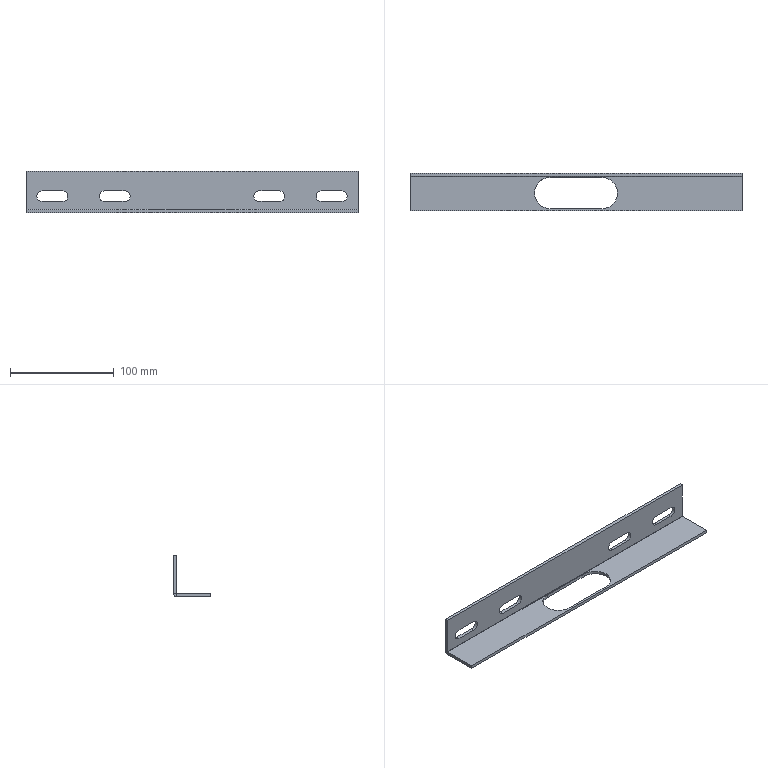Part | SolidWorks | features Cut 2, EdgeFlange 1, FlatPattern 1, SMBaseFlange 1, SheetMetal 1 | 1 solid | 35 faces | box 320 x 36 x 40 mm | volume 59416 mm3 | plane 22 | cylinder 13 | commonest cylinder face diameters 10 x8 30 x3 0.4 x1 6.4 x1
STEP:
#1=CARTESIAN_POINT('',(40.,-1.,-3.));
#2=VERTEX_POINT('',#1);
#3=CARTESIAN_POINT('',(25.,14.,-3.));
#4=VERTEX_POINT('',#3);
#5=CARTESIAN_POINT('',(25.,-1.,-3.));
#6=DIRECTION('',(0.,0.,1.));
#7=DIRECTION('',(1.,0.,0.));
#8=AXIS2_PLACEMENT_3D('',#5,#6,#7);
#9=CIRCLE('',#8,15.);
#10=EDGE_CURVE('',#2,#4,#9,.T.);
#11=ORIENTED_EDGE('',*,*,#10,.F.);
#12=CARTESIAN_POINT('',(40.,-1.,0.));
#13=VERTEX_POINT('',#12);
#14=CARTESIAN_POINT('',(40.,-1.,-10.));
#15=DIRECTION('',(0.,0.,1.));
#16=VECTOR('',#15,1000.);
#17=LINE('',#14,#16);
#18=EDGE_CURVE('',#2,#13,#17,.T.);
#19=ORIENTED_EDGE('',*,*,#18,.T.);
#20=CARTESIAN_POINT('',(25.,14.,0.));
#21=VERTEX_POINT('',#20);
#22=CARTESIAN_POINT('',(25.,-1.,0.));
#23=DIRECTION('',(0.,0.,1.));
#24=DIRECTION('',(1.,0.,0.));
#25=AXIS2_PLACEMENT_3D('',#22,#23,#24);
#26=CIRCLE('',#25,15.);
#27=EDGE_CURVE('',#13,#21,#26,.T.);
#28=ORIENTED_EDGE('',*,*,#27,.T.);
#29=CARTESIAN_POINT('',(25.,14.,-10.));
#30=DIRECTION('',(0.,0.,1.));
#31=VECTOR('',#30,1000.);
#32=LINE('',#29,#31);
#33=EDGE_CURVE('',#4,#21,#32,.T.);
#34=ORIENTED_EDGE('',*,*,#33,.F.);
#35=EDGE_LOOP('',(#11,#19,#28,#34));
#36=FACE_OUTER_BOUND('',#35,.T.);
#37=CARTESIAN_POINT('',(25.,-1.,-10.));
#38=DIRECTION('',(0.,0.,1.));
#39=DIRECTION('',(1.,0.,0.));
#40=AXIS2_PLACEMENT_3D('',#37,#38,#39);
#41=CYLINDRICAL_SURFACE('',#40,15.);
#42=ADVANCED_FACE('',(#36),#41,.F.);
#43=CARTESIAN_POINT('',(-160.,14.8,0.));
#44=VERTEX_POINT('',#43);
#45=CARTESIAN_POINT('',(-160.,-18.,0.));
#46=VERTEX_POINT('',#45);
#47=CARTESIAN_POINT('',(-160.,18.,0.));
#48=DIRECTION('',(0.,-1.,0.));
#49=VECTOR('',#48,1000.);
#50=LINE('',#47,#49);
#51=EDGE_CURVE('',#44,#46,#50,.T.);
#52=ORIENTED_EDGE('',*,*,#51,.F.);
#53=CARTESIAN_POINT('',(-160.,14.8,-3.));
#54=VERTEX_POINT('',#53);
#55=CARTESIAN_POINT('',(-160.,14.8,0.));
#56=DIRECTION('',(0.,0.,-1.));
#57=VECTOR('',#56,1000.);
#58=LINE('',#55,#57);
#59=EDGE_CURVE('',#44,#54,#58,.T.);
#60=ORIENTED_EDGE('',*,*,#59,.T.);
#61=CARTESIAN_POINT('',(-160.,-18.,-3.));
#62=VERTEX_POINT('',#61);
#63=CARTESIAN_POINT('',(-160.,18.,-3.));
#64=DIRECTION('',(0.,-1.,0.));
#65=VECTOR('',#64,1000.);
#66=LINE('',#63,#65);
#67=EDGE_CURVE('',#54,#62,#66,.T.);
#68=ORIENTED_EDGE('',*,*,#67,.T.);
#69=CARTESIAN_POINT('',(-160.,-18.,-3.));
#70=DIRECTION('',(0.,0.,1.));
#71=VECTOR('',#70,1000.);
#72=LINE('',#69,#71);
#73=EDGE_CURVE('',#62,#46,#72,.T.);
#74=ORIENTED_EDGE('',*,*,#73,.T.);
#75=EDGE_LOOP('',(#52,#60,#68,#74));
#76=FACE_OUTER_BOUND('',#75,.T.);
#77=CARTESIAN_POINT('',(-160.,18.,-3.));
#78=DIRECTION('',(-1.,0.,0.));
#79=DIRECTION('',(0.,0.,1.));
#80=AXIS2_PLACEMENT_3D('',#77,#78,#79);
#81=PLANE('',#80);
#82=ADVANCED_FACE('',(#76),#81,.T.);
#83=CARTESIAN_POINT('',(-25.,14.,-3.));
#84=VERTEX_POINT('',#83);
#85=CARTESIAN_POINT('',(0.,14.,-3.));
#86=DIRECTION('',(-1.,0.,0.));
#87=VECTOR('',#86,1000.);
#88=LINE('',#85,#87);
#89=EDGE_CURVE('',#4,#84,#88,.T.);
#90=ORIENTED_EDGE('',*,*,#89,.T.);
#91=CARTESIAN_POINT('',(-25.,-16.,-3.));
#92=VERTEX_POINT('',#91);
#93=CARTESIAN_POINT('',(-25.,-1.,-3.));
#94=DIRECTION('',(0.,0.,1.));
#95=DIRECTION('',(1.,0.,0.));
#96=AXIS2_PLACEMENT_3D('',#93,#94,#95);
#97=CIRCLE('',#96,15.);
#98=EDGE_CURVE('',#84,#92,#97,.T.);
#99=ORIENTED_EDGE('',*,*,#98,.T.);
#100=CARTESIAN_POINT('',(25.,-16.,-3.));
#101=VERTEX_POINT('',#100);
#102=CARTESIAN_POINT('',(0.,-16.,-3.));
#103=DIRECTION('',(1.,0.,0.));
#104=VECTOR('',#103,1000.);
#105=LINE('',#102,#104);
#106=EDGE_CURVE('',#92,#101,#105,.T.);
#107=ORIENTED_EDGE('',*,*,#106,.T.);
#108=CARTESIAN_POINT('',(25.,-1.,-3.));
#109=DIRECTION('',(0.,0.,1.));
#110=DIRECTION('',(1.,0.,0.));
#111=AXIS2_PLACEMENT_3D('',#108,#109,#110);
#112=CIRCLE('',#111,15.);
#113=EDGE_CURVE('',#101,#2,#112,.T.);
#114=ORIENTED_EDGE('',*,*,#113,.T.);
#115=ORIENTED_EDGE('',*,*,#10,.T.);
#116=EDGE_LOOP('',(#90,#99,#107,#114,#115));
#117=FACE_BOUND('',#116,.T.);
#118=CARTESIAN_POINT('',(160.,14.8,-3.));
#119=VERTEX_POINT('',#118);
#120=CARTESIAN_POINT('',(-160.,14.8,-3.));
#121=DIRECTION('',(1.,0.,0.));
#122=VECTOR('',#121,1000.);
#123=LINE('',#120,#122);
#124=EDGE_CURVE('',#54,#119,#123,.T.);
#125=ORIENTED_EDGE('',*,*,#124,.T.);
#126=CARTESIAN_POINT('',(160.,-18.,-3.));
#127=VERTEX_POINT('',#126);
#128=CARTESIAN_POINT('',(160.,18.,-3.));
#129=DIRECTION('',(0.,1.,0.));
#130=VECTOR('',#129,1000.);
#131=LINE('',#128,#130);
#132=EDGE_CURVE('',#127,#119,#131,.T.);
#133=ORIENTED_EDGE('',*,*,#132,.F.);
#134=CARTESIAN_POINT('',(-160.,-18.,-3.));
#135=DIRECTION('',(1.,0.,0.));
#136=VECTOR('',#135,1000.);
#137=LINE('',#134,#136);
#138=EDGE_CURVE('',#62,#127,#137,.T.);
#139=ORIENTED_EDGE('',*,*,#138,.F.);
#140=ORIENTED_EDGE('',*,*,#67,.F.);
#141=EDGE_LOOP('',(#125,#133,#139,#140));
#142=FACE_OUTER_BOUND('',#141,.T.);
#143=CARTESIAN_POINT('',(0.,0.,-3.));
#144=DIRECTION('',(0.,0.,1.));
#145=DIRECTION('',(1.,0.,0.));
#146=AXIS2_PLACEMENT_3D('',#143,#144,#145);
#147=PLANE('',#146);
#148=ADVANCED_FACE('',(#117,#142),#147,.F.);
#149=CARTESIAN_POINT('',(-25.,14.,0.));
#150=VERTEX_POINT('',#149);
#151=CARTESIAN_POINT('',(-25.,-16.,0.));
#152=VERTEX_POINT('',#151);
#153=CARTESIAN_POINT('',(-25.,-1.,0.));
#154=DIRECTION('',(0.,0.,1.));
#155=DIRECTION('',(1.,0.,0.));
#156=AXIS2_PLACEMENT_3D('',#153,#154,#155);
#157=CIRCLE('',#156,15.);
#158=EDGE_CURVE('',#150,#152,#157,.T.);
#159=ORIENTED_EDGE('',*,*,#158,.F.);
#160=CARTESIAN_POINT('',(-25.,14.,0.));
#161=DIRECTION('',(-1.,0.,0.));
#162=VECTOR('',#161,1000.);
#163=LINE('',#160,#162);
#164=EDGE_CURVE('',#21,#150,#163,.T.);
#165=ORIENTED_EDGE('',*,*,#164,.F.);
#166=ORIENTED_EDGE('',*,*,#27,.F.);
#167=CARTESIAN_POINT('',(25.,-16.,0.));
#168=VERTEX_POINT('',#167);
#169=CARTESIAN_POINT('',(25.,-1.,0.));
#170=DIRECTION('',(0.,0.,1.));
#171=DIRECTION('',(1.,0.,0.));
#172=AXIS2_PLACEMENT_3D('',#169,#170,#171);
#173=CIRCLE('',#172,15.);
#174=EDGE_CURVE('',#168,#13,#173,.T.);
#175=ORIENTED_EDGE('',*,*,#174,.F.);
#176=CARTESIAN_POINT('',(-25.,-16.,0.));
#177=DIRECTION('',(1.,0.,0.));
#178=VECTOR('',#177,1000.);
#179=LINE('',#176,#178);
#180=EDGE_CURVE('',#152,#168,#179,.T.);
#181=ORIENTED_EDGE('',*,*,#180,.F.);
#182=EDGE_LOOP('',(#159,#165,#166,#175,#181));
#183=FACE_BOUND('',#182,.T.);
#184=CARTESIAN_POINT('',(160.,-18.,0.));
#185=VERTEX_POINT('',#184);
#186=CARTESIAN_POINT('',(160.,14.8,0.));
#187=VERTEX_POINT('',#186);
#188=CARTESIAN_POINT('',(160.,18.,0.));
#189=DIRECTION('',(0.,1.,0.));
#190=VECTOR('',#189,1000.);
#191=LINE('',#188,#190);
#192=EDGE_CURVE('',#185,#187,#191,.T.);
#193=ORIENTED_EDGE('',*,*,#192,.T.);
#194=CARTESIAN_POINT('',(-160.,14.8,0.));
#195=DIRECTION('',(1.,0.,0.));
#196=VECTOR('',#195,1000.);
#197=LINE('',#194,#196);
#198=EDGE_CURVE('',#44,#187,#197,.T.);
#199=ORIENTED_EDGE('',*,*,#198,.F.);
#200=ORIENTED_EDGE('',*,*,#51,.T.);
#201=CARTESIAN_POINT('',(-160.,-18.,0.));
#202=DIRECTION('',(1.,0.,0.));
#203=VECTOR('',#202,1000.);
#204=LINE('',#201,#203);
#205=EDGE_CURVE('',#46,#185,#204,.T.);
#206=ORIENTED_EDGE('',*,*,#205,.T.);
#207=EDGE_LOOP('',(#193,#199,#200,#206));
#208=FACE_OUTER_BOUND('',#207,.T.);
#209=CARTESIAN_POINT('',(0.,0.,0.));
#210=DIRECTION('',(0.,0.,1.));
#211=DIRECTION('',(1.,0.,0.));
#212=AXIS2_PLACEMENT_3D('',#209,#210,#211);
#213=PLANE('',#212);
#214=ADVANCED_FACE('',(#183,#208),#213,.T.);
#215=CARTESIAN_POINT('',(160.,14.8,0.));
#216=DIRECTION('',(0.,0.,-1.));
#217=VECTOR('',#216,1000.);
#218=LINE('',#215,#217);
#219=EDGE_CURVE('',#187,#119,#218,.T.);
#220=ORIENTED_EDGE('',*,*,#219,.F.);
#221=ORIENTED_EDGE('',*,*,#192,.F.);
#222=CARTESIAN_POINT('',(160.,-18.,-3.));
#223=DIRECTION('',(0.,0.,1.));
#224=VECTOR('',#223,1000.);
#225=LINE('',#222,#224);
#226=EDGE_CURVE('',#127,#185,#225,.T.);
#227=ORIENTED_EDGE('',*,*,#226,.F.);
#228=ORIENTED_EDGE('',*,*,#132,.T.);
#229=EDGE_LOOP('',(#220,#221,#227,#228));
#230=FACE_OUTER_BOUND('',#229,.T.);
#231=CARTESIAN_POINT('',(160.,18.,-3.));
#232=DIRECTION('',(1.,0.,0.));
#233=DIRECTION('',(0.,0.,-1.));
#234=AXIS2_PLACEMENT_3D('',#231,#232,#233);
#235=PLANE('',#234);
#236=ADVANCED_FACE('',(#230),#235,.T.);
#237=ORIENTED_EDGE('',*,*,#205,.F.);
#238=ORIENTED_EDGE('',*,*,#73,.F.);
#239=ORIENTED_EDGE('',*,*,#138,.T.);
#240=ORIENTED_EDGE('',*,*,#226,.T.);
#241=EDGE_LOOP('',(#237,#238,#239,#240));
#242=FACE_OUTER_BOUND('',#241,.T.);
#243=CARTESIAN_POINT('',(-160.,-18.,-3.));
#244=DIRECTION('',(0.,-1.,0.));
#245=DIRECTION('',(0.,0.,-1.));
#246=AXIS2_PLACEMENT_3D('',#243,#244,#245);
#247=PLANE('',#246);
#248=ADVANCED_FACE('',(#242),#247,.T.);
#249=CARTESIAN_POINT('',(160.,15.,0.2));
#250=VERTEX_POINT('',#249);
#251=CARTESIAN_POINT('',(160.,18.,0.2));
#252=VERTEX_POINT('',#251);
#253=CARTESIAN_POINT('',(160.,18.,0.2));
#254=DIRECTION('',(0.,1.,0.));
#255=VECTOR('',#254,1000.);
#256=LINE('',#253,#255);
#257=EDGE_CURVE('',#250,#252,#256,.T.);
#258=ORIENTED_EDGE('',*,*,#257,.F.);
#259=CARTESIAN_POINT('',(160.,14.8,0.2));
#260=DIRECTION('',(1.,0.,0.));
#261=DIRECTION('',(0.,0.,1.));
#262=AXIS2_PLACEMENT_3D('',#259,#260,#261);
#263=CIRCLE('',#262,0.2);
#264=EDGE_CURVE('',#187,#250,#263,.T.);
#265=ORIENTED_EDGE('',*,*,#264,.F.);
#266=ORIENTED_EDGE('',*,*,#219,.T.);
#267=CARTESIAN_POINT('',(160.,14.8,0.2));
#268=DIRECTION('',(1.,0.,0.));
#269=DIRECTION('',(0.,0.,1.));
#270=AXIS2_PLACEMENT_3D('',#267,#268,#269);
#271=CIRCLE('',#270,3.2);
#272=EDGE_CURVE('',#119,#252,#271,.T.);
#273=ORIENTED_EDGE('',*,*,#272,.T.);
#274=EDGE_LOOP('',(#258,#265,#266,#273));
#275=FACE_OUTER_BOUND('',#274,.T.);
#276=CARTESIAN_POINT('',(160.,14.8,0.2));
#277=DIRECTION('',(1.,0.,0.));
#278=DIRECTION('',(0.,0.,-1.));
#279=AXIS2_PLACEMENT_3D('',#276,#277,#278);
#280=PLANE('',#279);
#281=ADVANCED_FACE('',(#275),#280,.T.);
#282=CARTESIAN_POINT('',(-160.,15.,0.2));
#283=VERTEX_POINT('',#282);
#284=CARTESIAN_POINT('',(-160.,14.8,0.2));
#285=DIRECTION('',(-1.,0.,0.));
#286=DIRECTION('',(0.,0.,1.));
#287=AXIS2_PLACEMENT_3D('',#284,#285,#286);
#288=CIRCLE('',#287,0.2);
#289=EDGE_CURVE('',#283,#44,#288,.T.);
#290=ORIENTED_EDGE('',*,*,#289,.F.);
#291=CARTESIAN_POINT('',(-160.,18.,0.2));
#292=VERTEX_POINT('',#291);
#293=CARTESIAN_POINT('',(-160.,15.,0.2));
#294=DIRECTION('',(0.,1.,0.));
#295=VECTOR('',#294,1000.);
#296=LINE('',#293,#295);
#297=EDGE_CURVE('',#283,#292,#296,.T.);
#298=ORIENTED_EDGE('',*,*,#297,.T.);
#299=CARTESIAN_POINT('',(-160.,14.8,0.2));
#300=DIRECTION('',(-1.,0.,0.));
#301=DIRECTION('',(0.,0.,1.));
#302=AXIS2_PLACEMENT_3D('',#299,#300,#301);
#303=CIRCLE('',#302,3.2);
#304=EDGE_CURVE('',#292,#54,#303,.T.);
#305=ORIENTED_EDGE('',*,*,#304,.T.);
#306=ORIENTED_EDGE('',*,*,#59,.F.);
#307=EDGE_LOOP('',(#290,#298,#305,#306));
#308=FACE_OUTER_BOUND('',#307,.T.);
#309=CARTESIAN_POINT('',(-160.,14.8,0.2));
#310=DIRECTION('',(1.,0.,0.));
#311=DIRECTION('',(0.,0.,-1.));
#312=AXIS2_PLACEMENT_3D('',#309,#310,#311);
#313=PLANE('',#312);
#314=ADVANCED_FACE('',(#308),#313,.F.);
#315=ORIENTED_EDGE('',*,*,#124,.F.);
#316=ORIENTED_EDGE('',*,*,#304,.F.);
#317=CARTESIAN_POINT('',(160.,18.,0.2));
#318=DIRECTION('',(1.,0.,0.));
#319=VECTOR('',#318,1000.);
#320=LINE('',#317,#319);
#321=EDGE_CURVE('',#292,#252,#320,.T.);
#322=ORIENTED_EDGE('',*,*,#321,.T.);
#323=ORIENTED_EDGE('',*,*,#272,.F.);
#324=EDGE_LOOP('',(#315,#316,#322,#323));
#325=FACE_OUTER_BOUND('',#324,.T.);
#326=CARTESIAN_POINT('',(-160.,14.8,0.2));
#327=DIRECTION('',(-1.,0.,0.));
#328=DIRECTION('',(0.,1.,0.));
#329=AXIS2_PLACEMENT_3D('',#326,#327,#328);
#330=CYLINDRICAL_SURFACE('',#329,3.2);
#331=ADVANCED_FACE('',(#325),#330,.T.);
#332=ORIENTED_EDGE('',*,*,#198,.T.);
#333=ORIENTED_EDGE('',*,*,#264,.T.);
#334=CARTESIAN_POINT('',(160.,15.,0.2));
#335=DIRECTION('',(-1.,0.,0.));
#336=VECTOR('',#335,1000.);
#337=LINE('',#334,#336);
#338=EDGE_CURVE('',#250,#283,#337,.T.);
#339=ORIENTED_EDGE('',*,*,#338,.T.);
#340=ORIENTED_EDGE('',*,*,#289,.T.);
#341=EDGE_LOOP('',(#332,#333,#339,#340));
#342=FACE_OUTER_BOUND('',#341,.T.);
#343=CARTESIAN_POINT('',(-160.,14.8,0.2));
#344=DIRECTION('',(-1.,0.,0.));
#345=DIRECTION('',(0.,1.,0.));
#346=AXIS2_PLACEMENT_3D('',#343,#344,#345);
#347=CYLINDRICAL_SURFACE('',#346,0.2);
#348=ADVANCED_FACE('',(#342),#347,.F.);
#349=ORIENTED_EDGE('',*,*,#257,.T.);
#350=CARTESIAN_POINT('',(160.,18.,37.));
#351=VERTEX_POINT('',#350);
#352=CARTESIAN_POINT('',(160.,18.,0.));
#353=DIRECTION('',(0.,0.,-1.));
#354=VECTOR('',#353,1000.);
#355=LINE('',#352,#354);
#356=EDGE_CURVE('',#351,#252,#355,.T.);
#357=ORIENTED_EDGE('',*,*,#356,.F.);
#358=CARTESIAN_POINT('',(160.,15.,37.));
#359=VERTEX_POINT('',#358);
#360=CARTESIAN_POINT('',(160.,18.,37.));
#361=DIRECTION('',(0.,-1.,0.));
#362=VECTOR('',#361,1000.);
#363=LINE('',#360,#362);
#364=EDGE_CURVE('',#351,#359,#363,.T.);
#365=ORIENTED_EDGE('',*,*,#364,.T.);
#366=CARTESIAN_POINT('',(160.,15.,0.));
#367=DIRECTION('',(0.,0.,-1.));
#368=VECTOR('',#367,1000.);
#369=LINE('',#366,#368);
#370=EDGE_CURVE('',#359,#250,#369,.T.);
#371=ORIENTED_EDGE('',*,*,#370,.T.);
#372=EDGE_LOOP('',(#349,#357,#365,#371));
#373=FACE_OUTER_BOUND('',#372,.T.);
#374=CARTESIAN_POINT('',(160.,18.,0.));
#375=DIRECTION('',(-1.,0.,0.));
#376=DIRECTION('',(0.,0.,1.));
#377=AXIS2_PLACEMENT_3D('',#374,#375,#376);
#378=PLANE('',#377);
#379=ADVANCED_FACE('',(#373),#378,.F.);
#380=ORIENTED_EDGE('',*,*,#297,.F.);
#381=CARTESIAN_POINT('',(-160.,15.,37.));
#382=VERTEX_POINT('',#381);
#383=CARTESIAN_POINT('',(-160.,15.,37.));
#384=DIRECTION('',(0.,0.,1.));
#385=VECTOR('',#384,1000.);
#386=LINE('',#383,#385);
#387=EDGE_CURVE('',#283,#382,#386,.T.);
#388=ORIENTED_EDGE('',*,*,#387,.T.);
#389=CARTESIAN_POINT('',(-160.,18.,37.));
#390=VERTEX_POINT('',#389);
#391=CARTESIAN_POINT('',(-160.,18.,37.));
#392=DIRECTION('',(0.,-1.,0.));
#393=VECTOR('',#392,1000.);
#394=LINE('',#391,#393);
#395=EDGE_CURVE('',#390,#382,#394,.T.);
#396=ORIENTED_EDGE('',*,*,#395,.F.);
#397=CARTESIAN_POINT('',(-160.,18.,0.));
#398=DIRECTION('',(0.,0.,1.));
#399=VECTOR('',#398,1000.);
#400=LINE('',#397,#399);
#401=EDGE_CURVE('',#292,#390,#400,.T.);
#402=ORIENTED_EDGE('',*,*,#401,.F.);
#403=EDGE_LOOP('',(#380,#388,#396,#402));
#404=FACE_OUTER_BOUND('',#403,.T.);
#405=CARTESIAN_POINT('',(-160.,18.,37.));
#406=DIRECTION('',(1.,0.,0.));
#407=DIRECTION('',(0.,0.,-1.));
#408=AXIS2_PLACEMENT_3D('',#405,#406,#407);
#409=PLANE('',#408);
#410=ADVANCED_FACE('',(#404),#409,.F.);
#411=CARTESIAN_POINT('',(-144.5,18.,18.));
#412=VERTEX_POINT('',#411);
#413=CARTESIAN_POINT('',(-124.5,18.,18.));
#414=VERTEX_POINT('',#413);
#415=CARTESIAN_POINT('',(-144.5,18.,18.));
#416=DIRECTION('',(1.,0.,0.));
#417=VECTOR('',#416,1000.);
#418=LINE('',#415,#417);
#419=EDGE_CURVE('',#412,#414,#418,.T.);
#420=ORIENTED_EDGE('',*,*,#419,.F.);
#421=CARTESIAN_POINT('',(-144.5,18.,8.));
#422=VERTEX_POINT('',#421);
#423=CARTESIAN_POINT('',(-144.5,18.,13.));
#424=DIRECTION('',(0.,1.,0.));
#425=DIRECTION('',(0.,0.,1.));
#426=AXIS2_PLACEMENT_3D('',#423,#424,#425);
#427=CIRCLE('',#426,5.);
#428=EDGE_CURVE('',#422,#412,#427,.T.);
#429=ORIENTED_EDGE('',*,*,#428,.F.);
#430=CARTESIAN_POINT('',(-124.5,18.,8.));
#431=VERTEX_POINT('',#430);
#432=CARTESIAN_POINT('',(-144.5,18.,8.));
#433=DIRECTION('',(-1.,0.,0.));
#434=VECTOR('',#433,1000.);
#435=LINE('',#432,#434);
#436=EDGE_CURVE('',#431,#422,#435,.T.);
#437=ORIENTED_EDGE('',*,*,#436,.F.);
#438=CARTESIAN_POINT('',(-124.5,18.,13.));
#439=DIRECTION('',(0.,1.,0.));
#440=DIRECTION('',(0.,0.,1.));
#441=AXIS2_PLACEMENT_3D('',#438,#439,#440);
#442=CIRCLE('',#441,5.);
#443=EDGE_CURVE('',#414,#431,#442,.T.);
#444=ORIENTED_EDGE('',*,*,#443,.F.);
#445=EDGE_LOOP('',(#420,#429,#437,#444));
#446=FACE_BOUND('',#445,.T.);
#447=CARTESIAN_POINT('',(-84.5,18.,18.));
#448=VERTEX_POINT('',#447);
#449=CARTESIAN_POINT('',(-64.5,18.,18.));
#450=VERTEX_POINT('',#449);
#451=CARTESIAN_POINT('',(-84.5,18.,18.));
#452=DIRECTION('',(1.,0.,0.));
#453=VECTOR('',#452,1000.);
#454=LINE('',#451,#453);
#455=EDGE_CURVE('',#448,#450,#454,.T.);
#456=ORIENTED_EDGE('',*,*,#455,.F.);
#457=CARTESIAN_POINT('',(-84.5,18.,8.));
#458=VERTEX_POINT('',#457);
#459=CARTESIAN_POINT('',(-84.5,18.,13.));
#460=DIRECTION('',(0.,1.,0.));
#461=DIRECTION('',(0.,0.,1.));
#462=AXIS2_PLACEMENT_3D('',#459,#460,#461);
#463=CIRCLE('',#462,5.);
#464=EDGE_CURVE('',#458,#448,#463,.T.);
#465=ORIENTED_EDGE('',*,*,#464,.F.);
#466=CARTESIAN_POINT('',(-64.5,18.,8.));
#467=VERTEX_POINT('',#466);
#468=CARTESIAN_POINT('',(-84.5,18.,8.));
#469=DIRECTION('',(-1.,0.,0.));
#470=VECTOR('',#469,1000.);
#471=LINE('',#468,#470);
#472=EDGE_CURVE('',#467,#458,#471,.T.);
#473=ORIENTED_EDGE('',*,*,#472,.F.);
#474=CARTESIAN_POINT('',(-64.5,18.,13.));
#475=DIRECTION('',(0.,1.,0.));
#476=DIRECTION('',(0.,0.,1.));
#477=AXIS2_PLACEMENT_3D('',#474,#475,#476);
#478=CIRCLE('',#477,5.);
#479=EDGE_CURVE('',#450,#467,#478,.T.);
#480=ORIENTED_EDGE('',*,*,#479,.F.);
#481=EDGE_LOOP('',(#456,#465,#473,#480));
#482=FACE_BOUND('',#481,.T.);
#483=CARTESIAN_POINT('',(84.5,18.,8.));
#484=VERTEX_POINT('',#483);
#485=CARTESIAN_POINT('',(64.5,18.,8.));
#486=VERTEX_POINT('',#485);
#487=CARTESIAN_POINT('',(84.5,18.,8.));
#488=DIRECTION('',(-1.,0.,0.));
#489=VECTOR('',#488,1000.);
#490=LINE('',#487,#489);
#491=EDGE_CURVE('',#484,#486,#490,.T.);
#492=ORIENTED_EDGE('',*,*,#491,.F.);
#493=CARTESIAN_POINT('',(84.5,18.,18.));
#494=VERTEX_POINT('',#493);
#495=CARTESIAN_POINT('',(84.5,18.,13.));
#496=DIRECTION('',(0.,1.,0.));
#497=DIRECTION('',(0.,0.,-1.));
#498=AXIS2_PLACEMENT_3D('',#495,#496,#497);
#499=CIRCLE('',#498,5.);
#500=EDGE_CURVE('',#494,#484,#499,.T.);
#501=ORIENTED_EDGE('',*,*,#500,.F.);
#502=CARTESIAN_POINT('',(64.5,18.,18.));
#503=VERTEX_POINT('',#502);
#504=CARTESIAN_POINT('',(84.5,18.,18.));
#505=DIRECTION('',(1.,0.,0.));
#506=VECTOR('',#505,1000.);
#507=LINE('',#504,#506);
#508=EDGE_CURVE('',#503,#494,#507,.T.);
#509=ORIENTED_EDGE('',*,*,#508,.F.);
#510=CARTESIAN_POINT('',(64.5,18.,13.));
#511=DIRECTION('',(0.,1.,0.));
#512=DIRECTION('',(0.,0.,-1.));
#513=AXIS2_PLACEMENT_3D('',#510,#511,#512);
#514=CIRCLE('',#513,5.);
#515=EDGE_CURVE('',#486,#503,#514,.T.);
#516=ORIENTED_EDGE('',*,*,#515,.F.);
#517=EDGE_LOOP('',(#492,#501,#509,#516));
#518=FACE_BOUND('',#517,.T.);
#519=CARTESIAN_POINT('',(144.5,18.,8.));
#520=VERTEX_POINT('',#519);
#521=CARTESIAN_POINT('',(124.5,18.,8.));
#522=VERTEX_POINT('',#521);
#523=CARTESIAN_POINT('',(144.5,18.,8.));
#524=DIRECTION('',(-1.,0.,0.));
#525=VECTOR('',#524,1000.);
#526=LINE('',#523,#525);
#527=EDGE_CURVE('',#520,#522,#526,.T.);
#528=ORIENTED_EDGE('',*,*,#527,.F.);
#529=CARTESIAN_POINT('',(144.5,18.,18.));
#530=VERTEX_POINT('',#529);
#531=CARTESIAN_POINT('',(144.5,18.,13.));
#532=DIRECTION('',(0.,1.,0.));
#533=DIRECTION('',(0.,0.,-1.));
#534=AXIS2_PLACEMENT_3D('',#531,#532,#533);
#535=CIRCLE('',#534,5.);
#536=EDGE_CURVE('',#530,#520,#535,.T.);
#537=ORIENTED_EDGE('',*,*,#536,.F.);
#538=CARTESIAN_POINT('',(124.5,18.,18.));
#539=VERTEX_POINT('',#538);
#540=CARTESIAN_POINT('',(144.5,18.,18.));
#541=DIRECTION('',(1.,0.,0.));
#542=VECTOR('',#541,1000.);
#543=LINE('',#540,#542);
#544=EDGE_CURVE('',#539,#530,#543,.T.);
#545=ORIENTED_EDGE('',*,*,#544,.F.);
#546=CARTESIAN_POINT('',(124.5,18.,13.));
#547=DIRECTION('',(0.,1.,0.));
#548=DIRECTION('',(0.,0.,-1.));
#549=AXIS2_PLACEMENT_3D('',#546,#547,#548);
#550=CIRCLE('',#549,5.);
#551=EDGE_CURVE('',#522,#539,#550,.T.);
#552=ORIENTED_EDGE('',*,*,#551,.F.);
#553=EDGE_LOOP('',(#528,#537,#545,#552));
#554=FACE_BOUND('',#553,.T.);
#555=ORIENTED_EDGE('',*,*,#321,.F.);
#556=ORIENTED_EDGE('',*,*,#401,.T.);
#557=CARTESIAN_POINT('',(0.,18.,37.));
#558=DIRECTION('',(1.,0.,0.));
#559=VECTOR('',#558,1000.);
#560=LINE('',#557,#559);
#561=EDGE_CURVE('',#390,#351,#560,.T.);
#562=ORIENTED_EDGE('',*,*,#561,.T.);
#563=ORIENTED_EDGE('',*,*,#356,.T.);
#564=EDGE_LOOP('',(#555,#556,#562,#563));
#565=FACE_OUTER_BOUND('',#564,.T.);
#566=CARTESIAN_POINT('',(0.,18.,0.));
#567=DIRECTION('',(0.,-1.,0.));
#568=DIRECTION('',(0.,0.,-1.));
#569=AXIS2_PLACEMENT_3D('',#566,#567,#568);
#570=PLANE('',#569);
#571=ADVANCED_FACE('',(#446,#482,#518,#554,#565),#570,.F.);
#572=CARTESIAN_POINT('',(-144.5,15.,18.));
#573=VERTEX_POINT('',#572);
#574=CARTESIAN_POINT('',(-144.5,15.,8.));
#575=VERTEX_POINT('',#574);
#576=CARTESIAN_POINT('',(-144.5,15.,13.));
#577=DIRECTION('',(0.,-1.,0.));
#578=DIRECTION('',(0.,0.,-1.));
#579=AXIS2_PLACEMENT_3D('',#576,#577,#578);
#580=CIRCLE('',#579,5.);
#581=EDGE_CURVE('',#573,#575,#580,.T.);
#582=ORIENTED_EDGE('',*,*,#581,.F.);
#583=CARTESIAN_POINT('',(-124.5,15.,18.));
#584=VERTEX_POINT('',#583);
#585=CARTESIAN_POINT('',(0.,15.,18.));
#586=DIRECTION('',(-1.,0.,0.));
#587=VECTOR('',#586,1000.);
#588=LINE('',#585,#587);
#589=EDGE_CURVE('',#584,#573,#588,.T.);
#590=ORIENTED_EDGE('',*,*,#589,.F.);
#591=CARTESIAN_POINT('',(-124.5,15.,8.));
#592=VERTEX_POINT('',#591);
#593=CARTESIAN_POINT('',(-124.5,15.,13.));
#594=DIRECTION('',(0.,-1.,0.));
#595=DIRECTION('',(0.,0.,-1.));
#596=AXIS2_PLACEMENT_3D('',#593,#594,#595);
#597=CIRCLE('',#596,5.);
#598=EDGE_CURVE('',#592,#584,#597,.T.);
#599=ORIENTED_EDGE('',*,*,#598,.F.);
#600=CARTESIAN_POINT('',(0.,15.,8.));
#601=DIRECTION('',(1.,0.,0.));
#602=VECTOR('',#601,1000.);
#603=LINE('',#600,#602);
#604=EDGE_CURVE('',#575,#592,#603,.T.);
#605=ORIENTED_EDGE('',*,*,#604,.F.);
#606=EDGE_LOOP('',(#582,#590,#599,#605));
#607=FACE_BOUND('',#606,.T.);
#608=CARTESIAN_POINT('',(-84.5,15.,18.));
#609=VERTEX_POINT('',#608);
#610=CARTESIAN_POINT('',(-84.5,15.,8.));
#611=VERTEX_POINT('',#610);
#612=CARTESIAN_POINT('',(-84.5,15.,13.));
#613=DIRECTION('',(0.,-1.,0.));
#614=DIRECTION('',(0.,0.,-1.));
#615=AXIS2_PLACEMENT_3D('',#612,#613,#614);
#616=CIRCLE('',#615,5.);
#617=EDGE_CURVE('',#609,#611,#616,.T.);
#618=ORIENTED_EDGE('',*,*,#617,.F.);
#619=CARTESIAN_POINT('',(-64.5,15.,18.));
#620=VERTEX_POINT('',#619);
#621=CARTESIAN_POINT('',(0.,15.,18.));
#622=DIRECTION('',(-1.,0.,0.));
#623=VECTOR('',#622,1000.);
#624=LINE('',#621,#623);
#625=EDGE_CURVE('',#620,#609,#624,.T.);
#626=ORIENTED_EDGE('',*,*,#625,.F.);
#627=CARTESIAN_POINT('',(-64.5,15.,8.));
#628=VERTEX_POINT('',#627);
#629=CARTESIAN_POINT('',(-64.5,15.,13.));
#630=DIRECTION('',(0.,-1.,0.));
#631=DIRECTION('',(0.,0.,-1.));
#632=AXIS2_PLACEMENT_3D('',#629,#630,#631);
#633=CIRCLE('',#632,5.);
#634=EDGE_CURVE('',#628,#620,#633,.T.);
#635=ORIENTED_EDGE('',*,*,#634,.F.);
#636=CARTESIAN_POINT('',(0.,15.,8.));
#637=DIRECTION('',(1.,0.,0.));
#638=VECTOR('',#637,1000.);
#639=LINE('',#636,#638);
#640=EDGE_CURVE('',#611,#628,#639,.T.);
#641=ORIENTED_EDGE('',*,*,#640,.F.);
#642=EDGE_LOOP('',(#618,#626,#635,#641));
#643=FACE_BOUND('',#642,.T.);
#644=CARTESIAN_POINT('',(84.5,15.,8.));
#645=VERTEX_POINT('',#644);
#646=CARTESIAN_POINT('',(84.5,15.,18.));
#647=VERTEX_POINT('',#646);
#648=CARTESIAN_POINT('',(84.5,15.,13.));
#649=DIRECTION('',(0.,-1.,0.));
#650=DIRECTION('',(0.,0.,-1.));
#651=AXIS2_PLACEMENT_3D('',#648,#649,#650);
#652=CIRCLE('',#651,5.);
#653=EDGE_CURVE('',#645,#647,#652,.T.);
#654=ORIENTED_EDGE('',*,*,#653,.F.);
#655=CARTESIAN_POINT('',(64.5,15.,8.));
#656=VERTEX_POINT('',#655);
#657=CARTESIAN_POINT('',(0.,15.,8.));
#658=DIRECTION('',(1.,0.,0.));
#659=VECTOR('',#658,1000.);
#660=LINE('',#657,#659);
#661=EDGE_CURVE('',#656,#645,#660,.T.);
#662=ORIENTED_EDGE('',*,*,#661,.F.);
#663=CARTESIAN_POINT('',(64.5,15.,18.));
#664=VERTEX_POINT('',#663);
#665=CARTESIAN_POINT('',(64.5,15.,13.));
#666=DIRECTION('',(0.,-1.,0.));
#667=DIRECTION('',(0.,0.,-1.));
#668=AXIS2_PLACEMENT_3D('',#665,#666,#667);
#669=CIRCLE('',#668,5.);
#670=EDGE_CURVE('',#664,#656,#669,.T.);
#671=ORIENTED_EDGE('',*,*,#670,.F.);
#672=CARTESIAN_POINT('',(0.,15.,18.));
#673=DIRECTION('',(-1.,0.,0.));
#674=VECTOR('',#673,1000.);
#675=LINE('',#672,#674);
#676=EDGE_CURVE('',#647,#664,#675,.T.);
#677=ORIENTED_EDGE('',*,*,#676,.F.);
#678=EDGE_LOOP('',(#654,#662,#671,#677));
#679=FACE_BOUND('',#678,.T.);
#680=CARTESIAN_POINT('',(144.5,15.,8.));
#681=VERTEX_POINT('',#680);
#682=CARTESIAN_POINT('',(144.5,15.,18.));
#683=VERTEX_POINT('',#682);
#684=CARTESIAN_POINT('',(144.5,15.,13.));
#685=DIRECTION('',(0.,-1.,0.));
#686=DIRECTION('',(0.,0.,-1.));
#687=AXIS2_PLACEMENT_3D('',#684,#685,#686);
#688=CIRCLE('',#687,5.);
#689=EDGE_CURVE('',#681,#683,#688,.T.);
#690=ORIENTED_EDGE('',*,*,#689,.F.);
#691=CARTESIAN_POINT('',(124.5,15.,8.));
#692=VERTEX_POINT('',#691);
#693=CARTESIAN_POINT('',(0.,15.,8.));
#694=DIRECTION('',(1.,0.,0.));
#695=VECTOR('',#694,1000.);
#696=LINE('',#693,#695);
#697=EDGE_CURVE('',#692,#681,#696,.T.);
#698=ORIENTED_EDGE('',*,*,#697,.F.);
#699=CARTESIAN_POINT('',(124.5,15.,18.));
#700=VERTEX_POINT('',#699);
#701=CARTESIAN_POINT('',(124.5,15.,13.));
#702=DIRECTION('',(0.,-1.,0.));
#703=DIRECTION('',(0.,0.,-1.));
#704=AXIS2_PLACEMENT_3D('',#701,#702,#703);
#705=CIRCLE('',#704,5.);
#706=EDGE_CURVE('',#700,#692,#705,.T.);
#707=ORIENTED_EDGE('',*,*,#706,.F.);
#708=CARTESIAN_POINT('',(0.,15.,18.));
#709=DIRECTION('',(-1.,0.,0.));
#710=VECTOR('',#709,1000.);
#711=LINE('',#708,#710);
#712=EDGE_CURVE('',#683,#700,#711,.T.);
#713=ORIENTED_EDGE('',*,*,#712,.F.);
#714=EDGE_LOOP('',(#690,#698,#707,#713));
#715=FACE_BOUND('',#714,.T.);
#716=ORIENTED_EDGE('',*,*,#387,.F.);
#717=ORIENTED_EDGE('',*,*,#338,.F.);
#718=ORIENTED_EDGE('',*,*,#370,.F.);
#719=CARTESIAN_POINT('',(160.,15.,37.));
#720=DIRECTION('',(1.,0.,0.));
#721=VECTOR('',#720,1000.);
#722=LINE('',#719,#721);
#723=EDGE_CURVE('',#382,#359,#722,.T.);
#724=ORIENTED_EDGE('',*,*,#723,.F.);
#725=EDGE_LOOP('',(#716,#717,#718,#724));
#726=FACE_OUTER_BOUND('',#725,.T.);
#727=CARTESIAN_POINT('',(0.,15.,0.));
#728=DIRECTION('',(0.,-1.,0.));
#729=DIRECTION('',(0.,0.,-1.));
#730=AXIS2_PLACEMENT_3D('',#727,#728,#729);
#731=PLANE('',#730);
#732=ADVANCED_FACE('',(#607,#643,#679,#715,#726),#731,.T.);
#733=ORIENTED_EDGE('',*,*,#723,.T.);
#734=ORIENTED_EDGE('',*,*,#364,.F.);
#735=ORIENTED_EDGE('',*,*,#561,.F.);
#736=ORIENTED_EDGE('',*,*,#395,.T.);
#737=EDGE_LOOP('',(#733,#734,#735,#736));
#738=FACE_OUTER_BOUND('',#737,.T.);
#739=CARTESIAN_POINT('',(160.,18.,37.));
#740=DIRECTION('',(0.,0.,-1.));
#741=DIRECTION('',(0.,1.,0.));
#742=AXIS2_PLACEMENT_3D('',#739,#740,#741);
#743=PLANE('',#742);
#744=ADVANCED_FACE('',(#738),#743,.F.);
#745=CARTESIAN_POINT('',(-25.,14.,-10.));
#746=DIRECTION('',(0.,0.,1.));
#747=VECTOR('',#746,1000.);
#748=LINE('',#745,#747);
#749=EDGE_CURVE('',#84,#150,#748,.T.);
#750=ORIENTED_EDGE('',*,*,#749,.T.);
#751=ORIENTED_EDGE('',*,*,#158,.T.);
#752=CARTESIAN_POINT('',(-25.,-16.,-10.));
#753=DIRECTION('',(0.,0.,1.));
#754=VECTOR('',#753,1000.);
#755=LINE('',#752,#754);
#756=EDGE_CURVE('',#92,#152,#755,.T.);
#757=ORIENTED_EDGE('',*,*,#756,.F.);
#758=ORIENTED_EDGE('',*,*,#98,.F.);
#759=EDGE_LOOP('',(#750,#751,#757,#758));
#760=FACE_OUTER_BOUND('',#759,.T.);
#761=CARTESIAN_POINT('',(-25.,-1.,-10.));
#762=DIRECTION('',(0.,0.,1.));
#763=DIRECTION('',(1.,0.,0.));
#764=AXIS2_PLACEMENT_3D('',#761,#762,#763);
#765=CYLINDRICAL_SURFACE('',#764,15.);
#766=ADVANCED_FACE('',(#760),#765,.F.);
#767=ORIENTED_EDGE('',*,*,#33,.T.);
#768=ORIENTED_EDGE('',*,*,#164,.T.);
#769=ORIENTED_EDGE('',*,*,#749,.F.);
#770=ORIENTED_EDGE('',*,*,#89,.F.);
#771=EDGE_LOOP('',(#767,#768,#769,#770));
#772=FACE_OUTER_BOUND('',#771,.T.);
#773=CARTESIAN_POINT('',(-25.,14.,-10.));
#774=DIRECTION('',(0.,1.,0.));
#775=DIRECTION('',(-1.,0.,0.));
#776=AXIS2_PLACEMENT_3D('',#773,#774,#775);
#777=PLANE('',#776);
#778=ADVANCED_FACE('',(#772),#777,.F.);
#779=ORIENTED_EDGE('',*,*,#18,.F.);
#780=ORIENTED_EDGE('',*,*,#113,.F.);
#781=CARTESIAN_POINT('',(25.,-16.,-10.));
#782=DIRECTION('',(0.,0.,1.));
#783=VECTOR('',#782,1000.);
#784=LINE('',#781,#783);
#785=EDGE_CURVE('',#101,#168,#784,.T.);
#786=ORIENTED_EDGE('',*,*,#785,.T.);
#787=ORIENTED_EDGE('',*,*,#174,.T.);
#788=EDGE_LOOP('',(#779,#780,#786,#787));
#789=FACE_OUTER_BOUND('',#788,.T.);
#790=CARTESIAN_POINT('',(25.,-1.,-10.));
#791=DIRECTION('',(0.,0.,1.));
#792=DIRECTION('',(1.,0.,0.));
#793=AXIS2_PLACEMENT_3D('',#790,#791,#792);
#794=CYLINDRICAL_SURFACE('',#793,15.);
#795=ADVANCED_FACE('',(#789),#794,.F.);
#796=ORIENTED_EDGE('',*,*,#756,.T.);
#797=ORIENTED_EDGE('',*,*,#180,.T.);
#798=ORIENTED_EDGE('',*,*,#785,.F.);
#799=ORIENTED_EDGE('',*,*,#106,.F.);
#800=EDGE_LOOP('',(#796,#797,#798,#799));
#801=FACE_OUTER_BOUND('',#800,.T.);
#802=CARTESIAN_POINT('',(-25.,-16.,-10.));
#803=DIRECTION('',(0.,-1.,0.));
#804=DIRECTION('',(1.,0.,0.));
#805=AXIS2_PLACEMENT_3D('',#802,#803,#804);
#806=PLANE('',#805);
#807=ADVANCED_FACE('',(#801),#806,.F.);
#808=ORIENTED_EDGE('',*,*,#689,.T.);
#809=CARTESIAN_POINT('',(144.5,8.,18.));
#810=DIRECTION('',(0.,1.,0.));
#811=VECTOR('',#810,1000.);
#812=LINE('',#809,#811);
#813=EDGE_CURVE('',#683,#530,#812,.T.);
#814=ORIENTED_EDGE('',*,*,#813,.T.);
#815=ORIENTED_EDGE('',*,*,#536,.T.);
#816=CARTESIAN_POINT('',(144.5,8.,8.));
#817=DIRECTION('',(0.,1.,0.));
#818=VECTOR('',#817,1000.);
#819=LINE('',#816,#818);
#820=EDGE_CURVE('',#681,#520,#819,.T.);
#821=ORIENTED_EDGE('',*,*,#820,.F.);
#822=EDGE_LOOP('',(#808,#814,#815,#821));
#823=FACE_OUTER_BOUND('',#822,.T.);
#824=CARTESIAN_POINT('',(144.5,8.,13.));
#825=DIRECTION('',(0.,1.,0.));
#826=DIRECTION('',(0.,0.,1.));
#827=AXIS2_PLACEMENT_3D('',#824,#825,#826);
#828=CYLINDRICAL_SURFACE('',#827,5.);
#829=ADVANCED_FACE('',(#823),#828,.F.);
#830=ORIENTED_EDGE('',*,*,#712,.T.);
#831=CARTESIAN_POINT('',(124.5,8.,18.));
#832=DIRECTION('',(0.,1.,0.));
#833=VECTOR('',#832,1000.);
#834=LINE('',#831,#833);
#835=EDGE_CURVE('',#700,#539,#834,.T.);
#836=ORIENTED_EDGE('',*,*,#835,.T.);
#837=ORIENTED_EDGE('',*,*,#544,.T.);
#838=ORIENTED_EDGE('',*,*,#813,.F.);
#839=EDGE_LOOP('',(#830,#836,#837,#838));
#840=FACE_OUTER_BOUND('',#839,.T.);
#841=CARTESIAN_POINT('',(144.5,8.,18.));
#842=DIRECTION('',(0.,0.,1.));
#843=DIRECTION('',(0.,-1.,0.));
#844=AXIS2_PLACEMENT_3D('',#841,#842,#843);
#845=PLANE('',#844);
#846=ADVANCED_FACE('',(#840),#845,.F.);
#847=ORIENTED_EDGE('',*,*,#706,.T.);
#848=CARTESIAN_POINT('',(124.5,8.,8.));
#849=DIRECTION('',(0.,1.,0.));
#850=VECTOR('',#849,1000.);
#851=LINE('',#848,#850);
#852=EDGE_CURVE('',#692,#522,#851,.T.);
#853=ORIENTED_EDGE('',*,*,#852,.T.);
#854=ORIENTED_EDGE('',*,*,#551,.T.);
#855=ORIENTED_EDGE('',*,*,#835,.F.);
#856=EDGE_LOOP('',(#847,#853,#854,#855));
#857=FACE_OUTER_BOUND('',#856,.T.);
#858=CARTESIAN_POINT('',(124.5,8.,13.));
#859=DIRECTION('',(0.,1.,0.));
#860=DIRECTION('',(0.,0.,1.));
#861=AXIS2_PLACEMENT_3D('',#858,#859,#860);
#862=CYLINDRICAL_SURFACE('',#861,5.);
#863=ADVANCED_FACE('',(#857),#862,.F.);
#864=ORIENTED_EDGE('',*,*,#697,.T.);
#865=ORIENTED_EDGE('',*,*,#820,.T.);
#866=ORIENTED_EDGE('',*,*,#527,.T.);
#867=ORIENTED_EDGE('',*,*,#852,.F.);
#868=EDGE_LOOP('',(#864,#865,#866,#867));
#869=FACE_OUTER_BOUND('',#868,.T.);
#870=CARTESIAN_POINT('',(144.5,8.,8.));
#871=DIRECTION('',(0.,0.,-1.));
#872=DIRECTION('',(0.,1.,0.));
#873=AXIS2_PLACEMENT_3D('',#870,#871,#872);
#874=PLANE('',#873);
#875=ADVANCED_FACE('',(#869),#874,.F.);
#876=ORIENTED_EDGE('',*,*,#653,.T.);
#877=CARTESIAN_POINT('',(84.5,8.,18.));
#878=DIRECTION('',(0.,1.,0.));
#879=VECTOR('',#878,1000.);
#880=LINE('',#877,#879);
#881=EDGE_CURVE('',#647,#494,#880,.T.);
#882=ORIENTED_EDGE('',*,*,#881,.T.);
#883=ORIENTED_EDGE('',*,*,#500,.T.);
#884=CARTESIAN_POINT('',(84.5,8.,8.));
#885=DIRECTION('',(0.,1.,0.));
#886=VECTOR('',#885,1000.);
#887=LINE('',#884,#886);
#888=EDGE_CURVE('',#645,#484,#887,.T.);
#889=ORIENTED_EDGE('',*,*,#888,.F.);
#890=EDGE_LOOP('',(#876,#882,#883,#889));
#891=FACE_OUTER_BOUND('',#890,.T.);
#892=CARTESIAN_POINT('',(84.5,8.,13.));
#893=DIRECTION('',(0.,1.,0.));
#894=DIRECTION('',(0.,0.,1.));
#895=AXIS2_PLACEMENT_3D('',#892,#893,#894);
#896=CYLINDRICAL_SURFACE('',#895,5.);
#897=ADVANCED_FACE('',(#891),#896,.F.);
#898=ORIENTED_EDGE('',*,*,#676,.T.);
#899=CARTESIAN_POINT('',(64.5,8.,18.));
#900=DIRECTION('',(0.,1.,0.));
#901=VECTOR('',#900,1000.);
#902=LINE('',#899,#901);
#903=EDGE_CURVE('',#664,#503,#902,.T.);
#904=ORIENTED_EDGE('',*,*,#903,.T.);
#905=ORIENTED_EDGE('',*,*,#508,.T.);
#906=ORIENTED_EDGE('',*,*,#881,.F.);
#907=EDGE_LOOP('',(#898,#904,#905,#906));
#908=FACE_OUTER_BOUND('',#907,.T.);
#909=CARTESIAN_POINT('',(84.5,8.,18.));
#910=DIRECTION('',(0.,0.,1.));
#911=DIRECTION('',(0.,-1.,0.));
#912=AXIS2_PLACEMENT_3D('',#909,#910,#911);
#913=PLANE('',#912);
#914=ADVANCED_FACE('',(#908),#913,.F.);
#915=ORIENTED_EDGE('',*,*,#670,.T.);
#916=CARTESIAN_POINT('',(64.5,8.,8.));
#917=DIRECTION('',(0.,1.,0.));
#918=VECTOR('',#917,1000.);
#919=LINE('',#916,#918);
#920=EDGE_CURVE('',#656,#486,#919,.T.);
#921=ORIENTED_EDGE('',*,*,#920,.T.);
#922=ORIENTED_EDGE('',*,*,#515,.T.);
#923=ORIENTED_EDGE('',*,*,#903,.F.);
#924=EDGE_LOOP('',(#915,#921,#922,#923));
#925=FACE_OUTER_BOUND('',#924,.T.);
#926=CARTESIAN_POINT('',(64.5,8.,13.));
#927=DIRECTION('',(0.,1.,0.));
#928=DIRECTION('',(0.,0.,1.));
#929=AXIS2_PLACEMENT_3D('',#926,#927,#928);
#930=CYLINDRICAL_SURFACE('',#929,5.);
#931=ADVANCED_FACE('',(#925),#930,.F.);
#932=ORIENTED_EDGE('',*,*,#661,.T.);
#933=ORIENTED_EDGE('',*,*,#888,.T.);
#934=ORIENTED_EDGE('',*,*,#491,.T.);
#935=ORIENTED_EDGE('',*,*,#920,.F.);
#936=EDGE_LOOP('',(#932,#933,#934,#935));
#937=FACE_OUTER_BOUND('',#936,.T.);
#938=CARTESIAN_POINT('',(84.5,8.,8.));
#939=DIRECTION('',(0.,0.,-1.));
#940=DIRECTION('',(0.,1.,0.));
#941=AXIS2_PLACEMENT_3D('',#938,#939,#940);
#942=PLANE('',#941);
#943=ADVANCED_FACE('',(#937),#942,.F.);
#944=ORIENTED_EDGE('',*,*,#617,.T.);
#945=CARTESIAN_POINT('',(-84.5,8.,8.));
#946=DIRECTION('',(0.,1.,0.));
#947=VECTOR('',#946,1000.);
#948=LINE('',#945,#947);
#949=EDGE_CURVE('',#611,#458,#948,.T.);
#950=ORIENTED_EDGE('',*,*,#949,.T.);
#951=ORIENTED_EDGE('',*,*,#464,.T.);
#952=CARTESIAN_POINT('',(-84.5,8.,18.));
#953=DIRECTION('',(0.,1.,0.));
#954=VECTOR('',#953,1000.);
#955=LINE('',#952,#954);
#956=EDGE_CURVE('',#609,#448,#955,.T.);
#957=ORIENTED_EDGE('',*,*,#956,.F.);
#958=EDGE_LOOP('',(#944,#950,#951,#957));
#959=FACE_OUTER_BOUND('',#958,.T.);
#960=CARTESIAN_POINT('',(-84.5,8.,13.));
#961=DIRECTION('',(0.,1.,0.));
#962=DIRECTION('',(0.,0.,1.));
#963=AXIS2_PLACEMENT_3D('',#960,#961,#962);
#964=CYLINDRICAL_SURFACE('',#963,5.);
#965=ADVANCED_FACE('',(#959),#964,.F.);
#966=ORIENTED_EDGE('',*,*,#640,.T.);
#967=CARTESIAN_POINT('',(-64.5,8.,8.));
#968=DIRECTION('',(0.,1.,0.));
#969=VECTOR('',#968,1000.);
#970=LINE('',#967,#969);
#971=EDGE_CURVE('',#628,#467,#970,.T.);
#972=ORIENTED_EDGE('',*,*,#971,.T.);
#973=ORIENTED_EDGE('',*,*,#472,.T.);
#974=ORIENTED_EDGE('',*,*,#949,.F.);
#975=EDGE_LOOP('',(#966,#972,#973,#974));
#976=FACE_OUTER_BOUND('',#975,.T.);
#977=CARTESIAN_POINT('',(-84.5,8.,8.));
#978=DIRECTION('',(0.,0.,-1.));
#979=DIRECTION('',(0.,1.,0.));
#980=AXIS2_PLACEMENT_3D('',#977,#978,#979);
#981=PLANE('',#980);
#982=ADVANCED_FACE('',(#976),#981,.F.);
#983=ORIENTED_EDGE('',*,*,#634,.T.);
#984=CARTESIAN_POINT('',(-64.5,8.,18.));
#985=DIRECTION('',(0.,1.,0.));
#986=VECTOR('',#985,1000.);
#987=LINE('',#984,#986);
#988=EDGE_CURVE('',#620,#450,#987,.T.);
#989=ORIENTED_EDGE('',*,*,#988,.T.);
#990=ORIENTED_EDGE('',*,*,#479,.T.);
#991=ORIENTED_EDGE('',*,*,#971,.F.);
#992=EDGE_LOOP('',(#983,#989,#990,#991));
#993=FACE_OUTER_BOUND('',#992,.T.);
#994=CARTESIAN_POINT('',(-64.5,8.,13.));
#995=DIRECTION('',(0.,1.,0.));
#996=DIRECTION('',(0.,0.,1.));
#997=AXIS2_PLACEMENT_3D('',#994,#995,#996);
#998=CYLINDRICAL_SURFACE('',#997,5.);
#999=ADVANCED_FACE('',(#993),#998,.F.);
#1000=ORIENTED_EDGE('',*,*,#625,.T.);
#1001=ORIENTED_EDGE('',*,*,#956,.T.);
#1002=ORIENTED_EDGE('',*,*,#455,.T.);
#1003=ORIENTED_EDGE('',*,*,#988,.F.);
#1004=EDGE_LOOP('',(#1000,#1001,#1002,#1003));
#1005=FACE_OUTER_BOUND('',#1004,.T.);
#1006=CARTESIAN_POINT('',(-84.5,8.,18.));
#1007=DIRECTION('',(0.,0.,1.));
#1008=DIRECTION('',(0.,-1.,0.));
#1009=AXIS2_PLACEMENT_3D('',#1006,#1007,#1008);
#1010=PLANE('',#1009);
#1011=ADVANCED_FACE('',(#1005),#1010,.F.);
#1012=ORIENTED_EDGE('',*,*,#581,.T.);
#1013=CARTESIAN_POINT('',(-144.5,8.,8.));
#1014=DIRECTION('',(0.,1.,0.));
#1015=VECTOR('',#1014,1000.);
#1016=LINE('',#1013,#1015);
#1017=EDGE_CURVE('',#575,#422,#1016,.T.);
#1018=ORIENTED_EDGE('',*,*,#1017,.T.);
#1019=ORIENTED_EDGE('',*,*,#428,.T.);
#1020=CARTESIAN_POINT('',(-144.5,8.,18.));
#1021=DIRECTION('',(0.,1.,0.));
#1022=VECTOR('',#1021,1000.);
#1023=LINE('',#1020,#1022);
#1024=EDGE_CURVE('',#573,#412,#1023,.T.);
#1025=ORIENTED_EDGE('',*,*,#1024,.F.);
#1026=EDGE_LOOP('',(#1012,#1018,#1019,#1025));
#1027=FACE_OUTER_BOUND('',#1026,.T.);
#1028=CARTESIAN_POINT('',(-144.5,8.,13.));
#1029=DIRECTION('',(0.,1.,0.));
#1030=DIRECTION('',(0.,0.,1.));
#1031=AXIS2_PLACEMENT_3D('',#1028,#1029,#1030);
#1032=CYLINDRICAL_SURFACE('',#1031,5.);
#1033=ADVANCED_FACE('',(#1027),#1032,.F.);
#1034=ORIENTED_EDGE('',*,*,#604,.T.);
#1035=CARTESIAN_POINT('',(-124.5,8.,8.));
#1036=DIRECTION('',(0.,1.,0.));
#1037=VECTOR('',#1036,1000.);
#1038=LINE('',#1035,#1037);
#1039=EDGE_CURVE('',#592,#431,#1038,.T.);
#1040=ORIENTED_EDGE('',*,*,#1039,.T.);
#1041=ORIENTED_EDGE('',*,*,#436,.T.);
#1042=ORIENTED_EDGE('',*,*,#1017,.F.);
#1043=EDGE_LOOP('',(#1034,#1040,#1041,#1042));
#1044=FACE_OUTER_BOUND('',#1043,.T.);
#1045=CARTESIAN_POINT('',(-144.5,8.,8.));
#1046=DIRECTION('',(0.,0.,-1.));
#1047=DIRECTION('',(0.,1.,0.));
#1048=AXIS2_PLACEMENT_3D('',#1045,#1046,#1047);
#1049=PLANE('',#1048);
#1050=ADVANCED_FACE('',(#1044),#1049,.F.);
#1051=ORIENTED_EDGE('',*,*,#598,.T.);
#1052=CARTESIAN_POINT('',(-124.5,8.,18.));
#1053=DIRECTION('',(0.,1.,0.));
#1054=VECTOR('',#1053,1000.);
#1055=LINE('',#1052,#1054);
#1056=EDGE_CURVE('',#584,#414,#1055,.T.);
#1057=ORIENTED_EDGE('',*,*,#1056,.T.);
#1058=ORIENTED_EDGE('',*,*,#443,.T.);
#1059=ORIENTED_EDGE('',*,*,#1039,.F.);
#1060=EDGE_LOOP('',(#1051,#1057,#1058,#1059));
#1061=FACE_OUTER_BOUND('',#1060,.T.);
#1062=CARTESIAN_POINT('',(-124.5,8.,13.));
#1063=DIRECTION('',(0.,1.,0.));
#1064=DIRECTION('',(0.,0.,1.));
#1065=AXIS2_PLACEMENT_3D('',#1062,#1063,#1064);
#1066=CYLINDRICAL_SURFACE('',#1065,5.);
#1067=ADVANCED_FACE('',(#1061),#1066,.F.);
#1068=ORIENTED_EDGE('',*,*,#589,.T.);
#1069=ORIENTED_EDGE('',*,*,#1024,.T.);
#1070=ORIENTED_EDGE('',*,*,#419,.T.);
#1071=ORIENTED_EDGE('',*,*,#1056,.F.);
#1072=EDGE_LOOP('',(#1068,#1069,#1070,#1071));
#1073=FACE_OUTER_BOUND('',#1072,.T.);
#1074=CARTESIAN_POINT('',(-144.5,8.,18.));
#1075=DIRECTION('',(0.,0.,1.));
#1076=DIRECTION('',(0.,-1.,0.));
#1077=AXIS2_PLACEMENT_3D('',#1074,#1075,#1076);
#1078=PLANE('',#1077);
#1079=ADVANCED_FACE('',(#1073),#1078,.F.);
#1080=CLOSED_SHELL('',(#42,#82,#148,#214,#236,#248,#281,#314,#331,#348,#379,#410,#571,#732,#744,#766,#778,#795,#807,#829,#846,#863,#875,#897,#914,#931,#943,#965,#982,#999,#1011,#1033,#1050,#1067,#1079));
#1081=MANIFOLD_SOLID_BREP('',#1080);
#1082=CARTESIAN_POINT('',(0.,0.,0.));
#1083=DIRECTION('',(0.,0.,1.));
#1084=DIRECTION('',(1.,0.,0.));
#1085=AXIS2_PLACEMENT_3D('',#1082,#1083,#1084);
#1086=(LENGTH_UNIT()NAMED_UNIT(*)SI_UNIT(.MILLI.,.METRE.));
#1087=UNCERTAINTY_MEASURE_WITH_UNIT(LENGTH_MEASURE(0.00001),#1086,'','');
#1088=(NAMED_UNIT(*)PLANE_ANGLE_UNIT()SI_UNIT($,.RADIAN.));
#1089=(NAMED_UNIT(*)SI_UNIT($,.STERADIAN.)SOLID_ANGLE_UNIT());
#1090=(GEOMETRIC_REPRESENTATION_CONTEXT(3)GLOBAL_UNCERTAINTY_ASSIGNED_CONTEXT((#1087))GLOBAL_UNIT_ASSIGNED_CONTEXT((#1086,#1088,#1089))REPRESENTATION_CONTEXT('',''));
#1091=ADVANCED_BREP_SHAPE_REPRESENTATION('',(#1081,#1085),#1090);